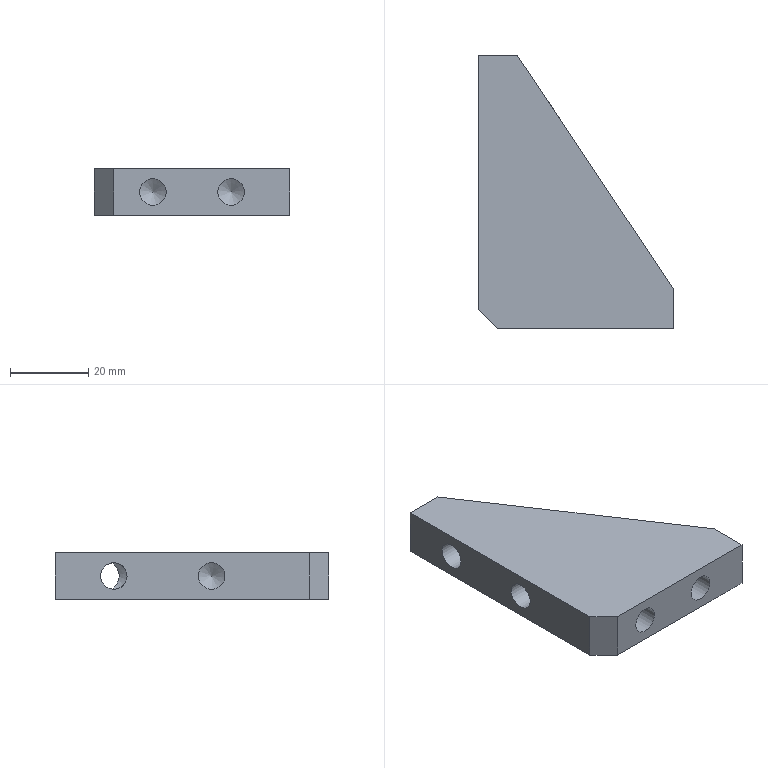Part | NX | features BREP 1 | 1 solid | 16 faces | box 50 x 70 x 12 mm | volume 24511 mm3 | plane 8 | cone 4 | cylinder 4 | commonest cylinder face diameters 6.8 x4
STEP:
#1=CARTESIAN_POINT('',(10.,70.,-6.));
#2=VERTEX_POINT('',#1);
#3=CARTESIAN_POINT('',(0.,70.,-6.));
#4=VERTEX_POINT('',#3);
#5=CARTESIAN_POINT('',(10.,70.,-6.));
#6=DIRECTION('',(-1.,0.,0.));
#7=VECTOR('',#6,1000.);
#8=LINE('',#5,#7);
#9=EDGE_CURVE('',#2,#4,#8,.T.);
#10=ORIENTED_EDGE('',*,*,#9,.T.);
#11=CARTESIAN_POINT('',(0.,70.,6.));
#12=VERTEX_POINT('',#11);
#13=CARTESIAN_POINT('',(0.,70.,6.));
#14=DIRECTION('',(0.,0.,-1.));
#15=VECTOR('',#14,1000.);
#16=LINE('',#13,#15);
#17=EDGE_CURVE('',#12,#4,#16,.T.);
#18=ORIENTED_EDGE('',*,*,#17,.F.);
#19=CARTESIAN_POINT('',(10.,70.,6.));
#20=VERTEX_POINT('',#19);
#21=CARTESIAN_POINT('',(10.,70.,6.));
#22=DIRECTION('',(-1.,0.,0.));
#23=VECTOR('',#22,1000.);
#24=LINE('',#21,#23);
#25=EDGE_CURVE('',#20,#12,#24,.T.);
#26=ORIENTED_EDGE('',*,*,#25,.F.);
#27=CARTESIAN_POINT('',(10.,70.,6.));
#28=DIRECTION('',(0.,0.,-1.));
#29=VECTOR('',#28,1000.);
#30=LINE('',#27,#29);
#31=EDGE_CURVE('',#20,#2,#30,.T.);
#32=ORIENTED_EDGE('',*,*,#31,.T.);
#33=EDGE_LOOP('',(#10,#18,#26,#32));
#34=FACE_BOUND('',#33,.T.);
#35=CARTESIAN_POINT('',(10.,70.,6.));
#36=DIRECTION('',(0.,-1.,0.));
#37=DIRECTION('',(0.,0.,1.));
#38=AXIS2_PLACEMENT_3D('',#35,#36,#37);
#39=PLANE('',#38);
#40=ADVANCED_FACE('',(#34),#39,.F.);
#41=CARTESIAN_POINT('',(0.,55.,3.4));
#42=VERTEX_POINT('',#41);
#43=CARTESIAN_POINT('',(0.,55.,0.));
#44=DIRECTION('',(-1.,0.,0.));
#45=DIRECTION('',(0.,0.,1.));
#46=AXIS2_PLACEMENT_3D('',#43,#44,#45);
#47=CIRCLE('',#46,3.4);
#48=EDGE_CURVE('',#42,#42,#47,.T.);
#49=ORIENTED_EDGE('',*,*,#48,.F.);
#50=EDGE_LOOP('',(#49));
#51=FACE_BOUND('',#50,.T.);
#52=CARTESIAN_POINT('',(0.,30.,3.4));
#53=VERTEX_POINT('',#52);
#54=CARTESIAN_POINT('',(0.,30.,0.));
#55=DIRECTION('',(-1.,0.,0.));
#56=DIRECTION('',(0.,0.,1.));
#57=AXIS2_PLACEMENT_3D('',#54,#55,#56);
#58=CIRCLE('',#57,3.4);
#59=EDGE_CURVE('',#53,#53,#58,.T.);
#60=ORIENTED_EDGE('',*,*,#59,.F.);
#61=EDGE_LOOP('',(#60));
#62=FACE_BOUND('',#61,.T.);
#63=CARTESIAN_POINT('',(0.,5.,-6.));
#64=VERTEX_POINT('',#63);
#65=CARTESIAN_POINT('',(0.,70.,-6.));
#66=DIRECTION('',(0.,-1.,0.));
#67=VECTOR('',#66,1000.);
#68=LINE('',#65,#67);
#69=EDGE_CURVE('',#4,#64,#68,.T.);
#70=ORIENTED_EDGE('',*,*,#69,.T.);
#71=CARTESIAN_POINT('',(0.,5.,6.));
#72=VERTEX_POINT('',#71);
#73=CARTESIAN_POINT('',(0.,5.,6.));
#74=DIRECTION('',(0.,0.,1.));
#75=VECTOR('',#74,1000.);
#76=LINE('',#73,#75);
#77=EDGE_CURVE('',#64,#72,#76,.T.);
#78=ORIENTED_EDGE('',*,*,#77,.T.);
#79=CARTESIAN_POINT('',(0.,70.,6.));
#80=DIRECTION('',(0.,-1.,0.));
#81=VECTOR('',#80,1000.);
#82=LINE('',#79,#81);
#83=EDGE_CURVE('',#12,#72,#82,.T.);
#84=ORIENTED_EDGE('',*,*,#83,.F.);
#85=ORIENTED_EDGE('',*,*,#17,.T.);
#86=EDGE_LOOP('',(#70,#78,#84,#85));
#87=FACE_BOUND('',#86,.T.);
#88=CARTESIAN_POINT('',(0.,70.,6.));
#89=DIRECTION('',(1.,0.,0.));
#90=DIRECTION('',(0.,-1.,0.));
#91=AXIS2_PLACEMENT_3D('',#88,#89,#90);
#92=PLANE('',#91);
#93=ADVANCED_FACE('',(#51,#62,#87),#92,.F.);
#94=CARTESIAN_POINT('',(15.,0.,-3.4));
#95=VERTEX_POINT('',#94);
#96=CARTESIAN_POINT('',(15.,0.,0.));
#97=DIRECTION('',(0.,-1.,0.));
#98=DIRECTION('',(0.,0.,-1.));
#99=AXIS2_PLACEMENT_3D('',#96,#97,#98);
#100=CIRCLE('',#99,3.4);
#101=EDGE_CURVE('',#95,#95,#100,.T.);
#102=ORIENTED_EDGE('',*,*,#101,.F.);
#103=EDGE_LOOP('',(#102));
#104=FACE_BOUND('',#103,.T.);
#105=CARTESIAN_POINT('',(35.,0.,-3.4));
#106=VERTEX_POINT('',#105);
#107=CARTESIAN_POINT('',(35.,0.,0.));
#108=DIRECTION('',(0.,-1.,0.));
#109=DIRECTION('',(0.,0.,-1.));
#110=AXIS2_PLACEMENT_3D('',#107,#108,#109);
#111=CIRCLE('',#110,3.4);
#112=EDGE_CURVE('',#106,#106,#111,.T.);
#113=ORIENTED_EDGE('',*,*,#112,.F.);
#114=EDGE_LOOP('',(#113));
#115=FACE_BOUND('',#114,.T.);
#116=CARTESIAN_POINT('',(5.,0.,6.));
#117=VERTEX_POINT('',#116);
#118=CARTESIAN_POINT('',(50.,0.,6.));
#119=VERTEX_POINT('',#118);
#120=CARTESIAN_POINT('',(0.,0.,6.));
#121=DIRECTION('',(1.,0.,0.));
#122=VECTOR('',#121,1000.);
#123=LINE('',#120,#122);
#124=EDGE_CURVE('',#117,#119,#123,.T.);
#125=ORIENTED_EDGE('',*,*,#124,.F.);
#126=CARTESIAN_POINT('',(5.,0.,-6.));
#127=VERTEX_POINT('',#126);
#128=CARTESIAN_POINT('',(5.,0.,6.));
#129=DIRECTION('',(0.,0.,-1.));
#130=VECTOR('',#129,1000.);
#131=LINE('',#128,#130);
#132=EDGE_CURVE('',#117,#127,#131,.T.);
#133=ORIENTED_EDGE('',*,*,#132,.T.);
#134=CARTESIAN_POINT('',(50.,0.,-6.));
#135=VERTEX_POINT('',#134);
#136=CARTESIAN_POINT('',(0.,0.,-6.));
#137=DIRECTION('',(1.,0.,0.));
#138=VECTOR('',#137,1000.);
#139=LINE('',#136,#138);
#140=EDGE_CURVE('',#127,#135,#139,.T.);
#141=ORIENTED_EDGE('',*,*,#140,.T.);
#142=CARTESIAN_POINT('',(50.,0.,6.));
#143=DIRECTION('',(0.,0.,-1.));
#144=VECTOR('',#143,1000.);
#145=LINE('',#142,#144);
#146=EDGE_CURVE('',#119,#135,#145,.T.);
#147=ORIENTED_EDGE('',*,*,#146,.F.);
#148=EDGE_LOOP('',(#125,#133,#141,#147));
#149=FACE_BOUND('',#148,.T.);
#150=CARTESIAN_POINT('',(0.,0.,6.));
#151=DIRECTION('',(0.,1.,0.));
#152=DIRECTION('',(0.,0.,-1.));
#153=AXIS2_PLACEMENT_3D('',#150,#151,#152);
#154=PLANE('',#153);
#155=ADVANCED_FACE('',(#104,#115,#149),#154,.F.);
#156=CARTESIAN_POINT('',(50.,10.,-6.));
#157=VERTEX_POINT('',#156);
#158=CARTESIAN_POINT('',(50.,0.,-6.));
#159=DIRECTION('',(0.,1.,0.));
#160=VECTOR('',#159,1000.);
#161=LINE('',#158,#160);
#162=EDGE_CURVE('',#135,#157,#161,.T.);
#163=ORIENTED_EDGE('',*,*,#162,.T.);
#164=CARTESIAN_POINT('',(50.,10.,6.));
#165=VERTEX_POINT('',#164);
#166=CARTESIAN_POINT('',(50.,10.,6.));
#167=DIRECTION('',(0.,0.,-1.));
#168=VECTOR('',#167,1000.);
#169=LINE('',#166,#168);
#170=EDGE_CURVE('',#165,#157,#169,.T.);
#171=ORIENTED_EDGE('',*,*,#170,.F.);
#172=CARTESIAN_POINT('',(50.,0.,6.));
#173=DIRECTION('',(0.,1.,0.));
#174=VECTOR('',#173,1000.);
#175=LINE('',#172,#174);
#176=EDGE_CURVE('',#119,#165,#175,.T.);
#177=ORIENTED_EDGE('',*,*,#176,.F.);
#178=ORIENTED_EDGE('',*,*,#146,.T.);
#179=EDGE_LOOP('',(#163,#171,#177,#178));
#180=FACE_BOUND('',#179,.T.);
#181=CARTESIAN_POINT('',(50.,0.,6.));
#182=DIRECTION('',(-1.,0.,0.));
#183=DIRECTION('',(0.,0.,-1.));
#184=AXIS2_PLACEMENT_3D('',#181,#182,#183);
#185=PLANE('',#184);
#186=ADVANCED_FACE('',(#180),#185,.F.);
#187=CARTESIAN_POINT('',(19.75,55.375,-3.379));
#188=VERTEX_POINT('',#187);
#189=CARTESIAN_POINT('',(19.75,55.375,3.379));
#190=VERTEX_POINT('',#189);
#191=CARTESIAN_POINT('',(19.75,55.375,-3.379));
#192=CARTESIAN_POINT('',(20.044,54.935,-2.936));
#193=CARTESIAN_POINT('',(20.6,54.099,-2.008));
#194=CARTESIAN_POINT('',(21.114,53.328,0.004513));
#195=CARTESIAN_POINT('',(20.6,54.1,2.006));
#196=CARTESIAN_POINT('',(20.043,54.935,2.937));
#197=CARTESIAN_POINT('',(19.75,55.375,3.379));
#198=B_SPLINE_CURVE_WITH_KNOTS('',3,(#191,#192,#193,#194,#195,#196,#197),.UNSPECIFIED.,.F.,.F.,(4,1,1,1,4),(0.,0.002059,0.004117,0.006176,0.008235),.UNSPECIFIED.);
#199=EDGE_CURVE('',#188,#190,#198,.T.);
#200=ORIENTED_EDGE('',*,*,#199,.T.);
#201=CARTESIAN_POINT('',(19.75,55.375,3.379));
#202=CARTESIAN_POINT('',(16.081,60.878,2.769));
#203=CARTESIAN_POINT('',(16.081,60.878,-2.769));
#204=CARTESIAN_POINT('',(19.75,55.375,-3.379));
#205=(BOUNDED_CURVE()B_SPLINE_CURVE(3,(#201,#202,#203,#204),.UNSPECIFIED.,.F.,.F.)B_SPLINE_CURVE_WITH_KNOTS((4,4),(0.,1.),.PIECEWISE_BEZIER_KNOTS.)CURVE()GEOMETRIC_REPRESENTATION_ITEM()RATIONAL_B_SPLINE_CURVE((1.,0.4069,0.4069,1.))REPRESENTATION_ITEM(''));
#206=EDGE_CURVE('',#190,#188,#205,.T.);
#207=ORIENTED_EDGE('',*,*,#206,.T.);
#208=EDGE_LOOP('',(#200,#207));
#209=FACE_BOUND('',#208,.T.);
#210=CARTESIAN_POINT('',(50.,10.,-6.));
#211=DIRECTION('',(-0.5547,0.8321,0.));
#212=VECTOR('',#211,1000.);
#213=LINE('',#210,#212);
#214=EDGE_CURVE('',#157,#2,#213,.T.);
#215=ORIENTED_EDGE('',*,*,#214,.T.);
#216=ORIENTED_EDGE('',*,*,#31,.F.);
#217=CARTESIAN_POINT('',(50.,10.,6.));
#218=DIRECTION('',(-0.5547,0.8321,0.));
#219=VECTOR('',#218,1000.);
#220=LINE('',#217,#219);
#221=EDGE_CURVE('',#165,#20,#220,.T.);
#222=ORIENTED_EDGE('',*,*,#221,.F.);
#223=ORIENTED_EDGE('',*,*,#170,.T.);
#224=EDGE_LOOP('',(#215,#216,#222,#223));
#225=FACE_BOUND('',#224,.T.);
#226=CARTESIAN_POINT('',(50.,10.,6.));
#227=DIRECTION('',(-0.8321,-0.5547,0.));
#228=DIRECTION('',(-0.5547,0.8321,0.));
#229=AXIS2_PLACEMENT_3D('',#226,#227,#228);
#230=PLANE('',#229);
#231=ADVANCED_FACE('',(#209,#225),#230,.F.);
#232=ORIENTED_EDGE('',*,*,#83,.T.);
#233=CARTESIAN_POINT('',(2.5,2.5,6.));
#234=DIRECTION('',(0.7071,-0.7071,0.));
#235=VECTOR('',#234,1000.);
#236=LINE('',#233,#235);
#237=EDGE_CURVE('',#72,#117,#236,.T.);
#238=ORIENTED_EDGE('',*,*,#237,.T.);
#239=ORIENTED_EDGE('',*,*,#124,.T.);
#240=ORIENTED_EDGE('',*,*,#176,.T.);
#241=ORIENTED_EDGE('',*,*,#221,.T.);
#242=ORIENTED_EDGE('',*,*,#25,.T.);
#243=EDGE_LOOP('',(#232,#238,#239,#240,#241,#242));
#244=FACE_BOUND('',#243,.T.);
#245=CARTESIAN_POINT('',(0.,0.,6.));
#246=DIRECTION('',(0.,0.,1.));
#247=DIRECTION('',(-1.,0.,0.));
#248=AXIS2_PLACEMENT_3D('',#245,#246,#247);
#249=PLANE('',#248);
#250=ADVANCED_FACE('',(#244),#249,.T.);
#251=ORIENTED_EDGE('',*,*,#140,.F.);
#252=CARTESIAN_POINT('',(5.,0.,-6.));
#253=DIRECTION('',(-0.7071,0.7071,0.));
#254=VECTOR('',#253,1000.);
#255=LINE('',#252,#254);
#256=EDGE_CURVE('',#127,#64,#255,.T.);
#257=ORIENTED_EDGE('',*,*,#256,.T.);
#258=ORIENTED_EDGE('',*,*,#69,.F.);
#259=ORIENTED_EDGE('',*,*,#9,.F.);
#260=ORIENTED_EDGE('',*,*,#214,.F.);
#261=ORIENTED_EDGE('',*,*,#162,.F.);
#262=EDGE_LOOP('',(#251,#257,#258,#259,#260,#261));
#263=FACE_BOUND('',#262,.T.);
#264=CARTESIAN_POINT('',(0.,0.,-6.));
#265=DIRECTION('',(0.,0.,1.));
#266=DIRECTION('',(-1.,0.,0.));
#267=AXIS2_PLACEMENT_3D('',#264,#265,#266);
#268=PLANE('',#267);
#269=ADVANCED_FACE('',(#263),#268,.F.);
#270=ORIENTED_EDGE('',*,*,#237,.F.);
#271=ORIENTED_EDGE('',*,*,#77,.F.);
#272=ORIENTED_EDGE('',*,*,#256,.F.);
#273=ORIENTED_EDGE('',*,*,#132,.F.);
#274=EDGE_LOOP('',(#270,#271,#272,#273));
#275=FACE_BOUND('',#274,.T.);
#276=CARTESIAN_POINT('',(5.,0.,6.));
#277=DIRECTION('',(0.7071,0.7071,0.));
#278=DIRECTION('',(0.,0.,1.));
#279=AXIS2_PLACEMENT_3D('',#276,#277,#278);
#280=PLANE('',#279);
#281=ADVANCED_FACE('',(#275),#280,.F.);
#282=CARTESIAN_POINT('',(21.793,30.,0.));
#283=VERTEX_POINT('',#282);
#284=VERTEX_LOOP('',#283);
#285=FACE_BOUND('',#284,.T.);
#286=CARTESIAN_POINT('',(19.75,30.,3.4));
#287=VERTEX_POINT('',#286);
#288=CARTESIAN_POINT('',(19.75,30.,0.));
#289=DIRECTION('',(-1.,0.,0.));
#290=DIRECTION('',(0.,0.,1.));
#291=AXIS2_PLACEMENT_3D('',#288,#289,#290);
#292=CIRCLE('',#291,3.4);
#293=EDGE_CURVE('',#287,#287,#292,.T.);
#294=ORIENTED_EDGE('',*,*,#293,.T.);
#295=EDGE_LOOP('',(#294));
#296=FACE_BOUND('',#295,.T.);
#297=CARTESIAN_POINT('',(19.75,30.,0.));
#298=DIRECTION('',(-1.,0.,0.));
#299=DIRECTION('',(0.,0.,-1.));
#300=AXIS2_PLACEMENT_3D('',#297,#298,#299);
#301=CONICAL_SURFACE('',#300,3.4,1.03);
#302=ADVANCED_FACE('',(#285,#296),#301,.F.);
#303=ORIENTED_EDGE('',*,*,#293,.F.);
#304=EDGE_LOOP('',(#303));
#305=FACE_BOUND('',#304,.T.);
#306=ORIENTED_EDGE('',*,*,#59,.T.);
#307=EDGE_LOOP('',(#306));
#308=FACE_BOUND('',#307,.T.);
#309=CARTESIAN_POINT('',(0.,30.,0.));
#310=DIRECTION('',(-1.,0.,0.));
#311=DIRECTION('',(0.,0.,-1.));
#312=AXIS2_PLACEMENT_3D('',#309,#310,#311);
#313=CYLINDRICAL_SURFACE('',#312,3.4);
#314=ADVANCED_FACE('',(#305,#308),#313,.F.);
#315=ORIENTED_EDGE('',*,*,#48,.T.);
#316=EDGE_LOOP('',(#315));
#317=FACE_BOUND('',#316,.T.);
#318=CARTESIAN_POINT('',(19.75,55.,0.));
#319=DIRECTION('',(-1.,0.,0.));
#320=DIRECTION('',(0.,0.,1.));
#321=AXIS2_PLACEMENT_3D('',#318,#319,#320);
#322=CIRCLE('',#321,3.4);
#323=EDGE_CURVE('',#188,#190,#322,.T.);
#324=ORIENTED_EDGE('',*,*,#323,.F.);
#325=ORIENTED_EDGE('',*,*,#206,.F.);
#326=EDGE_LOOP('',(#324,#325));
#327=FACE_BOUND('',#326,.T.);
#328=CARTESIAN_POINT('',(0.,55.,0.));
#329=DIRECTION('',(-1.,0.,0.));
#330=DIRECTION('',(0.,0.,-1.));
#331=AXIS2_PLACEMENT_3D('',#328,#329,#330);
#332=CYLINDRICAL_SURFACE('',#331,3.4);
#333=ADVANCED_FACE('',(#317,#327),#332,.F.);
#334=ORIENTED_EDGE('',*,*,#323,.T.);
#335=ORIENTED_EDGE('',*,*,#199,.F.);
#336=EDGE_LOOP('',(#334,#335));
#337=FACE_BOUND('',#336,.T.);
#338=CARTESIAN_POINT('',(19.75,55.,0.));
#339=DIRECTION('',(-1.,0.,0.));
#340=DIRECTION('',(0.,0.,-1.));
#341=AXIS2_PLACEMENT_3D('',#338,#339,#340);
#342=CONICAL_SURFACE('',#341,3.4,1.03);
#343=ADVANCED_FACE('',(#337),#342,.F.);
#344=CARTESIAN_POINT('',(35.,21.793,0.));
#345=VERTEX_POINT('',#344);
#346=VERTEX_LOOP('',#345);
#347=FACE_BOUND('',#346,.T.);
#348=CARTESIAN_POINT('',(35.,19.75,-3.4));
#349=VERTEX_POINT('',#348);
#350=CARTESIAN_POINT('',(35.,19.75,0.));
#351=DIRECTION('',(0.,-1.,0.));
#352=DIRECTION('',(0.,0.,-1.));
#353=AXIS2_PLACEMENT_3D('',#350,#351,#352);
#354=CIRCLE('',#353,3.4);
#355=EDGE_CURVE('',#349,#349,#354,.T.);
#356=ORIENTED_EDGE('',*,*,#355,.T.);
#357=EDGE_LOOP('',(#356));
#358=FACE_BOUND('',#357,.T.);
#359=CARTESIAN_POINT('',(35.,19.75,0.));
#360=DIRECTION('',(0.,-1.,0.));
#361=DIRECTION('',(0.,0.,1.));
#362=AXIS2_PLACEMENT_3D('',#359,#360,#361);
#363=CONICAL_SURFACE('',#362,3.4,1.03);
#364=ADVANCED_FACE('',(#347,#358),#363,.F.);
#365=ORIENTED_EDGE('',*,*,#355,.F.);
#366=EDGE_LOOP('',(#365));
#367=FACE_BOUND('',#366,.T.);
#368=ORIENTED_EDGE('',*,*,#112,.T.);
#369=EDGE_LOOP('',(#368));
#370=FACE_BOUND('',#369,.T.);
#371=CARTESIAN_POINT('',(35.,0.,0.));
#372=DIRECTION('',(0.,-1.,0.));
#373=DIRECTION('',(0.,0.,1.));
#374=AXIS2_PLACEMENT_3D('',#371,#372,#373);
#375=CYLINDRICAL_SURFACE('',#374,3.4);
#376=ADVANCED_FACE('',(#367,#370),#375,.F.);
#377=CARTESIAN_POINT('',(15.,21.793,0.));
#378=VERTEX_POINT('',#377);
#379=VERTEX_LOOP('',#378);
#380=FACE_BOUND('',#379,.T.);
#381=CARTESIAN_POINT('',(15.,19.75,-3.4));
#382=VERTEX_POINT('',#381);
#383=CARTESIAN_POINT('',(15.,19.75,0.));
#384=DIRECTION('',(0.,-1.,0.));
#385=DIRECTION('',(0.,0.,-1.));
#386=AXIS2_PLACEMENT_3D('',#383,#384,#385);
#387=CIRCLE('',#386,3.4);
#388=EDGE_CURVE('',#382,#382,#387,.T.);
#389=ORIENTED_EDGE('',*,*,#388,.T.);
#390=EDGE_LOOP('',(#389));
#391=FACE_BOUND('',#390,.T.);
#392=CARTESIAN_POINT('',(15.,19.75,0.));
#393=DIRECTION('',(0.,-1.,0.));
#394=DIRECTION('',(0.,0.,1.));
#395=AXIS2_PLACEMENT_3D('',#392,#393,#394);
#396=CONICAL_SURFACE('',#395,3.4,1.03);
#397=ADVANCED_FACE('',(#380,#391),#396,.F.);
#398=ORIENTED_EDGE('',*,*,#388,.F.);
#399=EDGE_LOOP('',(#398));
#400=FACE_BOUND('',#399,.T.);
#401=ORIENTED_EDGE('',*,*,#101,.T.);
#402=EDGE_LOOP('',(#401));
#403=FACE_BOUND('',#402,.T.);
#404=CARTESIAN_POINT('',(15.,0.,0.));
#405=DIRECTION('',(0.,-1.,0.));
#406=DIRECTION('',(0.,0.,1.));
#407=AXIS2_PLACEMENT_3D('',#404,#405,#406);
#408=CYLINDRICAL_SURFACE('',#407,3.4);
#409=ADVANCED_FACE('',(#400,#403),#408,.F.);
#410=CLOSED_SHELL('',(#40,#93,#155,#186,#231,#250,#269,#281,#302,#314,#333,#343,#364,#376,#397,#409));
#411=MANIFOLD_SOLID_BREP('',#410);
#412=(LENGTH_UNIT()NAMED_UNIT(*)SI_UNIT(.MILLI.,.METRE.));
#413=UNCERTAINTY_MEASURE_WITH_UNIT(LENGTH_MEASURE(0.0508),#412,'','');
#414=(NAMED_UNIT(*)PLANE_ANGLE_UNIT()SI_UNIT($,.RADIAN.));
#415=(NAMED_UNIT(*)SI_UNIT($,.STERADIAN.)SOLID_ANGLE_UNIT());
#416=(GEOMETRIC_REPRESENTATION_CONTEXT(3)GLOBAL_UNCERTAINTY_ASSIGNED_CONTEXT((#413))GLOBAL_UNIT_ASSIGNED_CONTEXT((#412,#414,#415))REPRESENTATION_CONTEXT('',''));
#417=ADVANCED_BREP_SHAPE_REPRESENTATION('',(#411),#416);